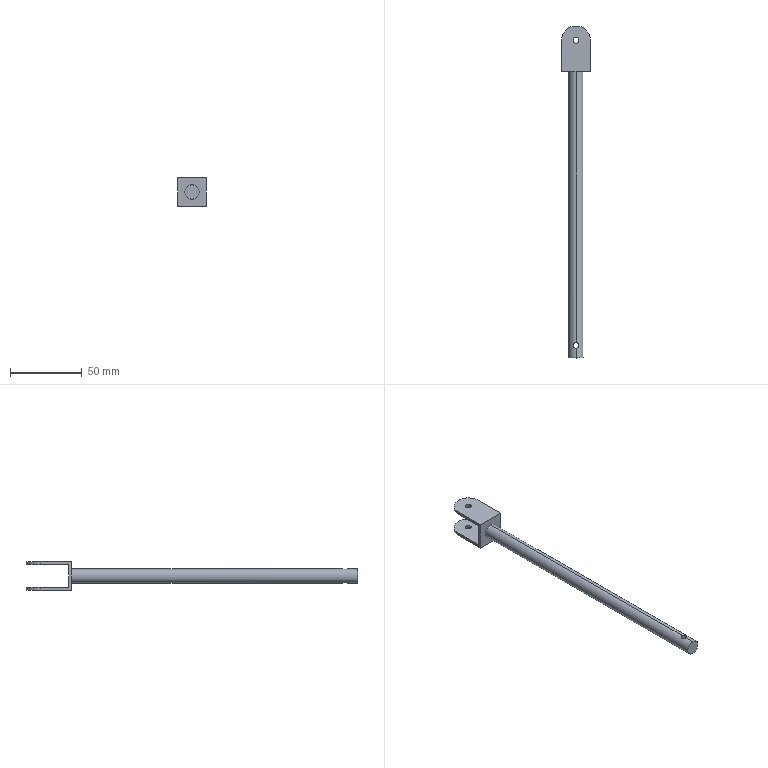Part | SolidWorks | features ICE 5, Extrusion 1 | 1 solid | 19 faces | box 20 x 232 x 20 mm | volume 18563 mm3 | cylinder 10 | plane 9 | commonest cylinder face diameters 4 x6 10 x2 20 x2
STEP:
#1=CARTESIAN_POINT('',(0.,-195.175,5.));
#2=VERTEX_POINT('',#1);
#3=CARTESIAN_POINT('',(2.,-193.175,4.583));
#4=VERTEX_POINT('',#3);
#5=CARTESIAN_POINT('',(0.,-195.175,5.));
#6=CARTESIAN_POINT('',(0.1337,-195.175,5.));
#7=CARTESIAN_POINT('',(0.2649,-195.162,4.995));
#8=CARTESIAN_POINT('',(0.5226,-195.11,4.974));
#9=CARTESIAN_POINT('',(0.6505,-195.071,4.959));
#10=CARTESIAN_POINT('',(0.8922,-194.97,4.921));
#11=CARTESIAN_POINT('',(1.007,-194.908,4.899));
#12=CARTESIAN_POINT('',(1.223,-194.763,4.849));
#13=CARTESIAN_POINT('',(1.324,-194.68,4.822));
#14=CARTESIAN_POINT('',(1.598,-194.405,4.742));
#15=CARTESIAN_POINT('',(1.746,-194.185,4.686));
#16=CARTESIAN_POINT('',(1.896,-193.825,4.627));
#17=CARTESIAN_POINT('',(1.935,-193.697,4.61));
#18=CARTESIAN_POINT('',(1.987,-193.438,4.588));
#19=CARTESIAN_POINT('',(2.,-193.307,4.583));
#20=CARTESIAN_POINT('',(2.,-193.175,4.583));
#21=B_SPLINE_CURVE_WITH_KNOTS('',3,(#5,#6,#7,#8,#9,#10,#11,#12,#13,#14,#15,#16,#17,#18,#19,#20),.UNSPECIFIED.,.F.,.F.,(4,2,2,2,2,2,2,4),(0.,0.0003951,0.0007903,0.001185,0.001581,0.002371,0.002766,0.003161),.UNSPECIFIED.);
#22=EDGE_CURVE('',#2,#4,#21,.T.);
#23=ORIENTED_EDGE('',*,*,#22,.T.);
#24=CARTESIAN_POINT('',(2.,-193.175,-4.583));
#25=VERTEX_POINT('',#24);
#26=CARTESIAN_POINT('',(2.,-193.175,30.5));
#27=DIRECTION('',(0.,0.,-1.));
#28=VECTOR('',#27,1000.);
#29=LINE('',#26,#28);
#30=EDGE_CURVE('',#4,#25,#29,.T.);
#31=ORIENTED_EDGE('',*,*,#30,.T.);
#32=CARTESIAN_POINT('',(0.,-195.175,-5.));
#33=VERTEX_POINT('',#32);
#34=CARTESIAN_POINT('',(2.,-193.175,-4.583));
#35=CARTESIAN_POINT('',(2.,-193.307,-4.583));
#36=CARTESIAN_POINT('',(1.987,-193.44,-4.588));
#37=CARTESIAN_POINT('',(1.935,-193.699,-4.611));
#38=CARTESIAN_POINT('',(1.896,-193.824,-4.627));
#39=CARTESIAN_POINT('',(1.795,-194.066,-4.667));
#40=CARTESIAN_POINT('',(1.733,-194.182,-4.691));
#41=CARTESIAN_POINT('',(1.589,-194.397,-4.742));
#42=CARTESIAN_POINT('',(1.506,-194.498,-4.769));
#43=CARTESIAN_POINT('',(1.322,-194.682,-4.823));
#44=CARTESIAN_POINT('',(1.222,-194.764,-4.85));
#45=CARTESIAN_POINT('',(1.007,-194.908,-4.899));
#46=CARTESIAN_POINT('',(0.8904,-194.971,-4.922));
#47=CARTESIAN_POINT('',(0.6487,-195.072,-4.959));
#48=CARTESIAN_POINT('',(0.5238,-195.11,-4.974));
#49=CARTESIAN_POINT('',(0.2659,-195.162,-4.995));
#50=CARTESIAN_POINT('',(0.1318,-195.175,-5.));
#51=CARTESIAN_POINT('',(0.,-195.175,-5.));
#52=B_SPLINE_CURVE_WITH_KNOTS('',3,(#34,#35,#36,#37,#38,#39,#40,#41,#42,#43,#44,#45,#46,#47,#48,#49,#50,#51),.UNSPECIFIED.,.F.,.F.,(4,2,2,2,2,2,2,2,4),(0.006319,0.006714,0.007109,0.007504,0.007898,0.008293,0.008688,0.009082,0.009477),.UNSPECIFIED.);
#53=EDGE_CURVE('',#25,#33,#52,.T.);
#54=ORIENTED_EDGE('',*,*,#53,.T.);
#55=CARTESIAN_POINT('',(-2.,-193.175,-4.583));
#56=VERTEX_POINT('',#55);
#57=CARTESIAN_POINT('',(0.,-195.175,-5.));
#58=CARTESIAN_POINT('',(-0.2635,-195.175,-5.));
#59=CARTESIAN_POINT('',(-0.5288,-195.122,-4.978));
#60=CARTESIAN_POINT('',(-0.8901,-194.971,-4.922));
#61=CARTESIAN_POINT('',(-1.007,-194.908,-4.899));
#62=CARTESIAN_POINT('',(-1.223,-194.763,-4.849));
#63=CARTESIAN_POINT('',(-1.322,-194.681,-4.823));
#64=CARTESIAN_POINT('',(-1.506,-194.498,-4.769));
#65=CARTESIAN_POINT('',(-1.589,-194.397,-4.741));
#66=CARTESIAN_POINT('',(-1.733,-194.182,-4.691));
#67=CARTESIAN_POINT('',(-1.794,-194.068,-4.667));
#68=CARTESIAN_POINT('',(-1.947,-193.704,-4.607));
#69=CARTESIAN_POINT('',(-2.,-193.442,-4.583));
#70=CARTESIAN_POINT('',(-2.,-193.175,-4.583));
#71=B_SPLINE_CURVE_WITH_KNOTS('',3,(#57,#58,#59,#60,#61,#62,#63,#64,#65,#66,#67,#68,#69,#70),.UNSPECIFIED.,.F.,.F.,(4,2,2,2,2,2,4),(0.009477,0.01027,0.01066,0.01106,0.01145,0.01184,0.01263),.UNSPECIFIED.);
#72=EDGE_CURVE('',#33,#56,#71,.T.);
#73=ORIENTED_EDGE('',*,*,#72,.T.);
#74=CARTESIAN_POINT('',(-2.,-193.175,4.583));
#75=VERTEX_POINT('',#74);
#76=CARTESIAN_POINT('',(-2.,-193.175,30.5));
#77=DIRECTION('',(0.,0.,-1.));
#78=VECTOR('',#77,1000.);
#79=LINE('',#76,#78);
#80=EDGE_CURVE('',#75,#56,#79,.T.);
#81=ORIENTED_EDGE('',*,*,#80,.F.);
#82=CARTESIAN_POINT('',(-2.,-193.175,4.583));
#83=CARTESIAN_POINT('',(-2.,-193.439,4.583));
#84=CARTESIAN_POINT('',(-1.946,-193.704,4.607));
#85=CARTESIAN_POINT('',(-1.796,-194.065,4.667));
#86=CARTESIAN_POINT('',(-1.733,-194.182,4.691));
#87=CARTESIAN_POINT('',(-1.588,-194.398,4.742));
#88=CARTESIAN_POINT('',(-1.506,-194.497,4.769));
#89=CARTESIAN_POINT('',(-1.323,-194.681,4.823));
#90=CARTESIAN_POINT('',(-1.222,-194.764,4.85));
#91=CARTESIAN_POINT('',(-1.007,-194.908,4.899));
#92=CARTESIAN_POINT('',(-0.8925,-194.97,4.921));
#93=CARTESIAN_POINT('',(-0.5272,-195.123,4.978));
#94=CARTESIAN_POINT('',(-0.2671,-195.175,5.));
#95=CARTESIAN_POINT('',(0.,-195.175,5.));
#96=B_SPLINE_CURVE_WITH_KNOTS('',3,(#82,#83,#84,#85,#86,#87,#88,#89,#90,#91,#92,#93,#94,#95),.UNSPECIFIED.,.F.,.F.,(4,2,2,2,2,2,4),(0.009478,0.01027,0.01066,0.01106,0.01145,0.01185,0.01264),.UNSPECIFIED.);
#97=EDGE_CURVE('',#75,#2,#96,.T.);
#98=ORIENTED_EDGE('',*,*,#97,.T.);
#99=EDGE_LOOP('',(#23,#31,#54,#73,#81,#98));
#100=FACE_OUTER_BOUND('',#99,.T.);
#101=CARTESIAN_POINT('',(0.,-193.175,30.5));
#102=DIRECTION('',(0.,0.,-1.));
#103=DIRECTION('',(-1.,0.,0.));
#104=AXIS2_PLACEMENT_3D('',#101,#102,#103);
#105=CYLINDRICAL_SURFACE('',#104,2.);
#106=ADVANCED_FACE('',(#100),#105,.F.);
#107=CARTESIAN_POINT('',(-2.,20.,10.));
#108=VERTEX_POINT('',#107);
#109=CARTESIAN_POINT('',(2.,20.,10.));
#110=VERTEX_POINT('',#109);
#111=CARTESIAN_POINT('',(0.,20.,10.));
#112=DIRECTION('',(0.,0.,1.));
#113=DIRECTION('',(1.,0.,0.));
#114=AXIS2_PLACEMENT_3D('',#111,#112,#113);
#115=CIRCLE('',#114,2.);
#116=EDGE_CURVE('',#108,#110,#115,.T.);
#117=ORIENTED_EDGE('',*,*,#116,.T.);
#118=CARTESIAN_POINT('',(2.,20.,8.));
#119=VERTEX_POINT('',#118);
#120=CARTESIAN_POINT('',(2.,20.,24.));
#121=DIRECTION('',(0.,0.,-1.));
#122=VECTOR('',#121,1000.);
#123=LINE('',#120,#122);
#124=EDGE_CURVE('',#110,#119,#123,.T.);
#125=ORIENTED_EDGE('',*,*,#124,.T.);
#126=CARTESIAN_POINT('',(-2.,20.,8.));
#127=VERTEX_POINT('',#126);
#128=CARTESIAN_POINT('',(0.,20.,8.));
#129=DIRECTION('',(0.,0.,-1.));
#130=DIRECTION('',(1.,0.,0.));
#131=AXIS2_PLACEMENT_3D('',#128,#129,#130);
#132=CIRCLE('',#131,2.);
#133=EDGE_CURVE('',#119,#127,#132,.T.);
#134=ORIENTED_EDGE('',*,*,#133,.T.);
#135=CARTESIAN_POINT('',(-2.,20.,24.));
#136=DIRECTION('',(0.,0.,-1.));
#137=VECTOR('',#136,1000.);
#138=LINE('',#135,#137);
#139=EDGE_CURVE('',#108,#127,#138,.T.);
#140=ORIENTED_EDGE('',*,*,#139,.F.);
#141=EDGE_LOOP('',(#117,#125,#134,#140));
#142=FACE_OUTER_BOUND('',#141,.T.);
#143=CARTESIAN_POINT('',(0.,20.,24.));
#144=DIRECTION('',(0.,0.,-1.));
#145=DIRECTION('',(-1.,0.,0.));
#146=AXIS2_PLACEMENT_3D('',#143,#144,#145);
#147=CYLINDRICAL_SURFACE('',#146,2.);
#148=ADVANCED_FACE('',(#142),#147,.F.);
#149=CARTESIAN_POINT('',(-2.,20.,-8.));
#150=VERTEX_POINT('',#149);
#151=CARTESIAN_POINT('',(2.,20.,-8.));
#152=VERTEX_POINT('',#151);
#153=CARTESIAN_POINT('',(0.,20.,-8.));
#154=DIRECTION('',(0.,0.,1.));
#155=DIRECTION('',(-1.,0.,0.));
#156=AXIS2_PLACEMENT_3D('',#153,#154,#155);
#157=CIRCLE('',#156,2.);
#158=EDGE_CURVE('',#150,#152,#157,.T.);
#159=ORIENTED_EDGE('',*,*,#158,.T.);
#160=CARTESIAN_POINT('',(2.,20.,-10.));
#161=VERTEX_POINT('',#160);
#162=CARTESIAN_POINT('',(2.,20.,24.));
#163=DIRECTION('',(0.,0.,-1.));
#164=VECTOR('',#163,1000.);
#165=LINE('',#162,#164);
#166=EDGE_CURVE('',#152,#161,#165,.T.);
#167=ORIENTED_EDGE('',*,*,#166,.T.);
#168=CARTESIAN_POINT('',(-2.,20.,-10.));
#169=VERTEX_POINT('',#168);
#170=CARTESIAN_POINT('',(0.,20.,-10.));
#171=DIRECTION('',(0.,0.,-1.));
#172=DIRECTION('',(-1.,0.,0.));
#173=AXIS2_PLACEMENT_3D('',#170,#171,#172);
#174=CIRCLE('',#173,2.);
#175=EDGE_CURVE('',#161,#169,#174,.T.);
#176=ORIENTED_EDGE('',*,*,#175,.T.);
#177=CARTESIAN_POINT('',(-2.,20.,24.));
#178=DIRECTION('',(0.,0.,-1.));
#179=VECTOR('',#178,1000.);
#180=LINE('',#177,#179);
#181=EDGE_CURVE('',#150,#169,#180,.T.);
#182=ORIENTED_EDGE('',*,*,#181,.F.);
#183=EDGE_LOOP('',(#159,#167,#176,#182));
#184=FACE_OUTER_BOUND('',#183,.T.);
#185=CARTESIAN_POINT('',(0.,20.,24.));
#186=DIRECTION('',(0.,0.,-1.));
#187=DIRECTION('',(-1.,0.,0.));
#188=AXIS2_PLACEMENT_3D('',#185,#186,#187);
#189=CYLINDRICAL_SURFACE('',#188,2.);
#190=ADVANCED_FACE('',(#184),#189,.F.);
#191=CARTESIAN_POINT('',(0.,-202.,-5.));
#192=VERTEX_POINT('',#191);
#193=CARTESIAN_POINT('',(0.,-202.,5.));
#194=VERTEX_POINT('',#193);
#195=CARTESIAN_POINT('',(0.,-202.,0.));
#196=DIRECTION('',(0.,-1.,0.));
#197=DIRECTION('',(0.,0.,-1.));
#198=AXIS2_PLACEMENT_3D('',#195,#196,#197);
#199=CIRCLE('',#198,5.);
#200=EDGE_CURVE('',#192,#194,#199,.T.);
#201=ORIENTED_EDGE('',*,*,#200,.F.);
#202=CARTESIAN_POINT('',(0.,-202.,-5.));
#203=DIRECTION('',(0.,1.,0.));
#204=VECTOR('',#203,1000.);
#205=LINE('',#202,#204);
#206=EDGE_CURVE('',#192,#33,#205,.T.);
#207=ORIENTED_EDGE('',*,*,#206,.T.);
#208=ORIENTED_EDGE('',*,*,#53,.F.);
#209=CARTESIAN_POINT('',(0.,-191.175,-5.));
#210=VERTEX_POINT('',#209);
#211=CARTESIAN_POINT('',(0.,-191.175,-5.));
#212=CARTESIAN_POINT('',(0.1321,-191.175,-5.));
#213=CARTESIAN_POINT('',(0.266,-191.189,-4.995));
#214=CARTESIAN_POINT('',(0.5238,-191.241,-4.974));
#215=CARTESIAN_POINT('',(0.6494,-191.279,-4.959));
#216=CARTESIAN_POINT('',(0.8932,-191.381,-4.921));
#217=CARTESIAN_POINT('',(1.008,-191.443,-4.899));
#218=CARTESIAN_POINT('',(1.223,-191.587,-4.849));
#219=CARTESIAN_POINT('',(1.325,-191.671,-4.822));
#220=CARTESIAN_POINT('',(1.507,-191.854,-4.768));
#221=CARTESIAN_POINT('',(1.589,-191.954,-4.741));
#222=CARTESIAN_POINT('',(1.734,-192.17,-4.69));
#223=CARTESIAN_POINT('',(1.796,-192.286,-4.666));
#224=CARTESIAN_POINT('',(1.946,-192.647,-4.607));
#225=CARTESIAN_POINT('',(2.,-192.912,-4.583));
#226=CARTESIAN_POINT('',(2.,-193.175,-4.583));
#227=B_SPLINE_CURVE_WITH_KNOTS('',3,(#211,#212,#213,#214,#215,#216,#217,#218,#219,#220,#221,#222,#223,#224,#225,#226),.UNSPECIFIED.,.F.,.F.,(4,2,2,2,2,2,2,4),(0.003161,0.003556,0.00395,0.004345,0.00474,0.005135,0.00553,0.006319),.UNSPECIFIED.);
#228=EDGE_CURVE('',#210,#25,#227,.T.);
#229=ORIENTED_EDGE('',*,*,#228,.F.);
#230=CARTESIAN_POINT('',(0.,-2.,-5.));
#231=VERTEX_POINT('',#230);
#232=CARTESIAN_POINT('',(0.,-202.,-5.));
#233=DIRECTION('',(0.,1.,0.));
#234=VECTOR('',#233,1000.);
#235=LINE('',#232,#234);
#236=EDGE_CURVE('',#210,#231,#235,.T.);
#237=ORIENTED_EDGE('',*,*,#236,.T.);
#238=CARTESIAN_POINT('',(0.,-2.,5.));
#239=VERTEX_POINT('',#238);
#240=CARTESIAN_POINT('',(0.,-2.,0.));
#241=DIRECTION('',(0.,-1.,0.));
#242=DIRECTION('',(0.,0.,-1.));
#243=AXIS2_PLACEMENT_3D('',#240,#241,#242);
#244=CIRCLE('',#243,5.);
#245=EDGE_CURVE('',#231,#239,#244,.T.);
#246=ORIENTED_EDGE('',*,*,#245,.T.);
#247=CARTESIAN_POINT('',(0.,-191.175,5.));
#248=VERTEX_POINT('',#247);
#249=CARTESIAN_POINT('',(0.,-202.,5.));
#250=DIRECTION('',(0.,1.,0.));
#251=VECTOR('',#250,1000.);
#252=LINE('',#249,#251);
#253=EDGE_CURVE('',#248,#239,#252,.T.);
#254=ORIENTED_EDGE('',*,*,#253,.F.);
#255=CARTESIAN_POINT('',(2.,-193.175,4.583));
#256=CARTESIAN_POINT('',(2.,-193.043,4.583));
#257=CARTESIAN_POINT('',(1.987,-192.909,4.588));
#258=CARTESIAN_POINT('',(1.935,-192.652,4.611));
#259=CARTESIAN_POINT('',(1.896,-192.526,4.627));
#260=CARTESIAN_POINT('',(1.795,-192.283,4.667));
#261=CARTESIAN_POINT('',(1.733,-192.168,4.691));
#262=CARTESIAN_POINT('',(1.588,-191.953,4.742));
#263=CARTESIAN_POINT('',(1.505,-191.852,4.769));
#264=CARTESIAN_POINT('',(1.322,-191.669,4.823));
#265=CARTESIAN_POINT('',(1.222,-191.587,4.85));
#266=CARTESIAN_POINT('',(1.006,-191.442,4.899));
#267=CARTESIAN_POINT('',(0.8895,-191.379,4.922));
#268=CARTESIAN_POINT('',(0.5289,-191.229,4.978));
#269=CARTESIAN_POINT('',(0.2632,-191.175,5.));
#270=CARTESIAN_POINT('',(0.,-191.175,5.));
#271=B_SPLINE_CURVE_WITH_KNOTS('',3,(#255,#256,#257,#258,#259,#260,#261,#262,#263,#264,#265,#266,#267,#268,#269,#270),.UNSPECIFIED.,.F.,.F.,(4,2,2,2,2,2,2,4),(0.003161,0.003556,0.003951,0.004346,0.00474,0.005135,0.00553,0.00632),.UNSPECIFIED.);
#272=EDGE_CURVE('',#4,#248,#271,.T.);
#273=ORIENTED_EDGE('',*,*,#272,.F.);
#274=ORIENTED_EDGE('',*,*,#22,.F.);
#275=CARTESIAN_POINT('',(0.,-202.,5.));
#276=DIRECTION('',(0.,1.,0.));
#277=VECTOR('',#276,1000.);
#278=LINE('',#275,#277);
#279=EDGE_CURVE('',#194,#2,#278,.T.);
#280=ORIENTED_EDGE('',*,*,#279,.F.);
#281=EDGE_LOOP('',(#201,#207,#208,#229,#237,#246,#254,#273,#274,#280));
#282=FACE_OUTER_BOUND('',#281,.T.);
#283=CARTESIAN_POINT('',(0.,-202.,0.));
#284=DIRECTION('',(0.,1.,0.));
#285=DIRECTION('',(0.,0.,1.));
#286=AXIS2_PLACEMENT_3D('',#283,#284,#285);
#287=CYLINDRICAL_SURFACE('',#286,5.);
#288=ADVANCED_FACE('',(#282),#287,.T.);
#289=ORIENTED_EDGE('',*,*,#206,.F.);
#290=CARTESIAN_POINT('',(0.,-202.,0.));
#291=DIRECTION('',(0.,-1.,0.));
#292=DIRECTION('',(0.,0.,-1.));
#293=AXIS2_PLACEMENT_3D('',#290,#291,#292);
#294=CIRCLE('',#293,5.);
#295=EDGE_CURVE('',#194,#192,#294,.T.);
#296=ORIENTED_EDGE('',*,*,#295,.F.);
#297=ORIENTED_EDGE('',*,*,#279,.T.);
#298=ORIENTED_EDGE('',*,*,#97,.F.);
#299=CARTESIAN_POINT('',(0.,-191.175,5.));
#300=CARTESIAN_POINT('',(-0.1316,-191.175,5.));
#301=CARTESIAN_POINT('',(-0.2649,-191.189,4.995));
#302=CARTESIAN_POINT('',(-0.5241,-191.241,4.974));
#303=CARTESIAN_POINT('',(-0.6493,-191.279,4.959));
#304=CARTESIAN_POINT('',(-0.8913,-191.38,4.921));
#305=CARTESIAN_POINT('',(-1.008,-191.443,4.899));
#306=CARTESIAN_POINT('',(-1.223,-191.587,4.849));
#307=CARTESIAN_POINT('',(-1.323,-191.67,4.823));
#308=CARTESIAN_POINT('',(-1.508,-191.855,4.768));
#309=CARTESIAN_POINT('',(-1.589,-191.954,4.741));
#310=CARTESIAN_POINT('',(-1.733,-192.169,4.691));
#311=CARTESIAN_POINT('',(-1.796,-192.285,4.667));
#312=CARTESIAN_POINT('',(-1.897,-192.527,4.627));
#313=CARTESIAN_POINT('',(-1.935,-192.652,4.611));
#314=CARTESIAN_POINT('',(-1.987,-192.909,4.588));
#315=CARTESIAN_POINT('',(-2.,-193.043,4.583));
#316=CARTESIAN_POINT('',(-2.,-193.175,4.583));
#317=B_SPLINE_CURVE_WITH_KNOTS('',3,(#299,#300,#301,#302,#303,#304,#305,#306,#307,#308,#309,#310,#311,#312,#313,#314,#315,#316),.UNSPECIFIED.,.F.,.F.,(4,2,2,2,2,2,2,2,4),(0.00632,0.006715,0.007109,0.007504,0.007899,0.008294,0.008688,0.009083,0.009478),.UNSPECIFIED.);
#318=EDGE_CURVE('',#248,#75,#317,.T.);
#319=ORIENTED_EDGE('',*,*,#318,.F.);
#320=ORIENTED_EDGE('',*,*,#253,.T.);
#321=CARTESIAN_POINT('',(0.,-2.,0.));
#322=DIRECTION('',(0.,-1.,0.));
#323=DIRECTION('',(0.,0.,-1.));
#324=AXIS2_PLACEMENT_3D('',#321,#322,#323);
#325=CIRCLE('',#324,5.);
#326=EDGE_CURVE('',#239,#231,#325,.T.);
#327=ORIENTED_EDGE('',*,*,#326,.T.);
#328=ORIENTED_EDGE('',*,*,#236,.F.);
#329=CARTESIAN_POINT('',(-2.,-193.175,-4.583));
#330=CARTESIAN_POINT('',(-2.,-193.042,-4.583));
#331=CARTESIAN_POINT('',(-1.987,-192.91,-4.588));
#332=CARTESIAN_POINT('',(-1.935,-192.653,-4.61));
#333=CARTESIAN_POINT('',(-1.896,-192.525,-4.627));
#334=CARTESIAN_POINT('',(-1.795,-192.284,-4.667));
#335=CARTESIAN_POINT('',(-1.734,-192.169,-4.691));
#336=CARTESIAN_POINT('',(-1.588,-191.953,-4.742));
#337=CARTESIAN_POINT('',(-1.505,-191.852,-4.769));
#338=CARTESIAN_POINT('',(-1.231,-191.578,-4.85));
#339=CARTESIAN_POINT('',(-1.01,-191.43,-4.903));
#340=CARTESIAN_POINT('',(-0.6497,-191.279,-4.959));
#341=CARTESIAN_POINT('',(-0.522,-191.24,-4.974));
#342=CARTESIAN_POINT('',(-0.263,-191.188,-4.995));
#343=CARTESIAN_POINT('',(-0.1322,-191.175,-5.));
#344=CARTESIAN_POINT('',(0.,-191.175,-5.));
#345=B_SPLINE_CURVE_WITH_KNOTS('',3,(#329,#330,#331,#332,#333,#334,#335,#336,#337,#338,#339,#340,#341,#342,#343,#344),.UNSPECIFIED.,.F.,.F.,(4,2,2,2,2,2,2,4),(0.,0.0003951,0.0007902,0.001185,0.00158,0.002371,0.002766,0.003161),.UNSPECIFIED.);
#346=EDGE_CURVE('',#56,#210,#345,.T.);
#347=ORIENTED_EDGE('',*,*,#346,.F.);
#348=ORIENTED_EDGE('',*,*,#72,.F.);
#349=EDGE_LOOP('',(#289,#296,#297,#298,#319,#320,#327,#328,#347,#348));
#350=FACE_OUTER_BOUND('',#349,.T.);
#351=CARTESIAN_POINT('',(0.,-202.,0.));
#352=DIRECTION('',(0.,1.,0.));
#353=DIRECTION('',(0.,0.,1.));
#354=AXIS2_PLACEMENT_3D('',#351,#352,#353);
#355=CYLINDRICAL_SURFACE('',#354,5.);
#356=ADVANCED_FACE('',(#350),#355,.T.);
#357=CARTESIAN_POINT('',(-10.,0.,8.));
#358=VERTEX_POINT('',#357);
#359=CARTESIAN_POINT('',(-10.,0.,-8.));
#360=VERTEX_POINT('',#359);
#361=CARTESIAN_POINT('',(-10.,0.,-10.));
#362=DIRECTION('',(0.,0.,-1.));
#363=VECTOR('',#362,1000.);
#364=LINE('',#361,#363);
#365=EDGE_CURVE('',#358,#360,#364,.T.);
#366=ORIENTED_EDGE('',*,*,#365,.F.);
#367=CARTESIAN_POINT('',(10.,0.,8.));
#368=VERTEX_POINT('',#367);
#369=CARTESIAN_POINT('',(-10.,0.,8.));
#370=DIRECTION('',(1.,0.,0.));
#371=VECTOR('',#370,1000.);
#372=LINE('',#369,#371);
#373=EDGE_CURVE('',#358,#368,#372,.T.);
#374=ORIENTED_EDGE('',*,*,#373,.T.);
#375=CARTESIAN_POINT('',(10.,0.,-8.));
#376=VERTEX_POINT('',#375);
#377=CARTESIAN_POINT('',(10.,0.,-10.));
#378=DIRECTION('',(0.,0.,1.));
#379=VECTOR('',#378,1000.);
#380=LINE('',#377,#379);
#381=EDGE_CURVE('',#376,#368,#380,.T.);
#382=ORIENTED_EDGE('',*,*,#381,.F.);
#383=CARTESIAN_POINT('',(-10.,0.,-8.));
#384=DIRECTION('',(-1.,0.,0.));
#385=VECTOR('',#384,1000.);
#386=LINE('',#383,#385);
#387=EDGE_CURVE('',#376,#360,#386,.T.);
#388=ORIENTED_EDGE('',*,*,#387,.T.);
#389=EDGE_LOOP('',(#366,#374,#382,#388));
#390=FACE_OUTER_BOUND('',#389,.T.);
#391=CARTESIAN_POINT('',(0.,0.,0.));
#392=DIRECTION('',(0.,1.,0.));
#393=DIRECTION('',(0.,0.,1.));
#394=AXIS2_PLACEMENT_3D('',#391,#392,#393);
#395=PLANE('',#394);
#396=ADVANCED_FACE('',(#390),#395,.T.);
#397=CARTESIAN_POINT('',(-10.,20.,-8.));
#398=VERTEX_POINT('',#397);
#399=CARTESIAN_POINT('',(-10.,20.,-10.));
#400=VERTEX_POINT('',#399);
#401=CARTESIAN_POINT('',(-10.,20.,10.));
#402=DIRECTION('',(0.,0.,-1.));
#403=VECTOR('',#402,1000.);
#404=LINE('',#401,#403);
#405=EDGE_CURVE('',#398,#400,#404,.T.);
#406=ORIENTED_EDGE('',*,*,#405,.F.);
#407=CARTESIAN_POINT('',(10.,20.,-8.));
#408=VERTEX_POINT('',#407);
#409=CARTESIAN_POINT('',(0.,20.,-8.));
#410=DIRECTION('',(0.,0.,-1.));
#411=DIRECTION('',(-1.,0.,0.));
#412=AXIS2_PLACEMENT_3D('',#409,#410,#411);
#413=CIRCLE('',#412,10.);
#414=EDGE_CURVE('',#398,#408,#413,.T.);
#415=ORIENTED_EDGE('',*,*,#414,.T.);
#416=CARTESIAN_POINT('',(10.,20.,-10.));
#417=VERTEX_POINT('',#416);
#418=CARTESIAN_POINT('',(10.,20.,10.));
#419=DIRECTION('',(0.,0.,-1.));
#420=VECTOR('',#419,1000.);
#421=LINE('',#418,#420);
#422=EDGE_CURVE('',#408,#417,#421,.T.);
#423=ORIENTED_EDGE('',*,*,#422,.T.);
#424=CARTESIAN_POINT('',(0.,20.,-10.));
#425=DIRECTION('',(0.,0.,1.));
#426=DIRECTION('',(1.,0.,0.));
#427=AXIS2_PLACEMENT_3D('',#424,#425,#426);
#428=CIRCLE('',#427,10.);
#429=EDGE_CURVE('',#417,#400,#428,.T.);
#430=ORIENTED_EDGE('',*,*,#429,.T.);
#431=EDGE_LOOP('',(#406,#415,#423,#430));
#432=FACE_OUTER_BOUND('',#431,.T.);
#433=CARTESIAN_POINT('',(0.,20.,10.));
#434=DIRECTION('',(0.,0.,-1.));
#435=DIRECTION('',(-1.,0.,0.));
#436=AXIS2_PLACEMENT_3D('',#433,#434,#435);
#437=CYLINDRICAL_SURFACE('',#436,10.);
#438=ADVANCED_FACE('',(#432),#437,.T.);
#439=CARTESIAN_POINT('',(-10.,-2.,-10.));
#440=VERTEX_POINT('',#439);
#441=CARTESIAN_POINT('',(-10.,20.,-10.));
#442=DIRECTION('',(0.,-1.,0.));
#443=VECTOR('',#442,1000.);
#444=LINE('',#441,#443);
#445=EDGE_CURVE('',#400,#440,#444,.T.);
#446=ORIENTED_EDGE('',*,*,#445,.T.);
#447=CARTESIAN_POINT('',(-10.,-2.,10.));
#448=VERTEX_POINT('',#447);
#449=CARTESIAN_POINT('',(-10.,-2.,-10.));
#450=DIRECTION('',(0.,0.,-1.));
#451=VECTOR('',#450,1000.);
#452=LINE('',#449,#451);
#453=EDGE_CURVE('',#448,#440,#452,.T.);
#454=ORIENTED_EDGE('',*,*,#453,.F.);
#455=CARTESIAN_POINT('',(-10.,20.,10.));
#456=VERTEX_POINT('',#455);
#457=CARTESIAN_POINT('',(-10.,-2.,10.));
#458=DIRECTION('',(0.,1.,0.));
#459=VECTOR('',#458,1000.);
#460=LINE('',#457,#459);
#461=EDGE_CURVE('',#448,#456,#460,.T.);
#462=ORIENTED_EDGE('',*,*,#461,.T.);
#463=CARTESIAN_POINT('',(-10.,20.,8.));
#464=VERTEX_POINT('',#463);
#465=CARTESIAN_POINT('',(-10.,20.,10.));
#466=DIRECTION('',(0.,0.,-1.));
#467=VECTOR('',#466,1000.);
#468=LINE('',#465,#467);
#469=EDGE_CURVE('',#456,#464,#468,.T.);
#470=ORIENTED_EDGE('',*,*,#469,.T.);
#471=CARTESIAN_POINT('',(-10.,20.,8.));
#472=DIRECTION('',(0.,-1.,0.));
#473=VECTOR('',#472,1000.);
#474=LINE('',#471,#473);
#475=EDGE_CURVE('',#464,#358,#474,.T.);
#476=ORIENTED_EDGE('',*,*,#475,.T.);
#477=ORIENTED_EDGE('',*,*,#365,.T.);
#478=CARTESIAN_POINT('',(-10.,20.,-8.));
#479=DIRECTION('',(0.,1.,0.));
#480=VECTOR('',#479,1000.);
#481=LINE('',#478,#480);
#482=EDGE_CURVE('',#360,#398,#481,.T.);
#483=ORIENTED_EDGE('',*,*,#482,.T.);
#484=ORIENTED_EDGE('',*,*,#405,.T.);
#485=EDGE_LOOP('',(#446,#454,#462,#470,#476,#477,#483,#484));
#486=FACE_OUTER_BOUND('',#485,.T.);
#487=CARTESIAN_POINT('',(-10.,20.,10.));
#488=DIRECTION('',(1.,0.,0.));
#489=DIRECTION('',(0.,1.,0.));
#490=AXIS2_PLACEMENT_3D('',#487,#488,#489);
#491=PLANE('',#490);
#492=ADVANCED_FACE('',(#486),#491,.F.);
#493=ORIENTED_EDGE('',*,*,#422,.F.);
#494=CARTESIAN_POINT('',(10.,0.,-8.));
#495=DIRECTION('',(0.,-1.,0.));
#496=VECTOR('',#495,1000.);
#497=LINE('',#494,#496);
#498=EDGE_CURVE('',#408,#376,#497,.T.);
#499=ORIENTED_EDGE('',*,*,#498,.T.);
#500=ORIENTED_EDGE('',*,*,#381,.T.);
#501=CARTESIAN_POINT('',(10.,20.,8.));
#502=VERTEX_POINT('',#501);
#503=CARTESIAN_POINT('',(10.,0.,8.));
#504=DIRECTION('',(0.,1.,0.));
#505=VECTOR('',#504,1000.);
#506=LINE('',#503,#505);
#507=EDGE_CURVE('',#368,#502,#506,.T.);
#508=ORIENTED_EDGE('',*,*,#507,.T.);
#509=CARTESIAN_POINT('',(10.,20.,10.));
#510=VERTEX_POINT('',#509);
#511=CARTESIAN_POINT('',(10.,20.,10.));
#512=DIRECTION('',(0.,0.,-1.));
#513=VECTOR('',#512,1000.);
#514=LINE('',#511,#513);
#515=EDGE_CURVE('',#510,#502,#514,.T.);
#516=ORIENTED_EDGE('',*,*,#515,.F.);
#517=CARTESIAN_POINT('',(10.,-2.,10.));
#518=VERTEX_POINT('',#517);
#519=CARTESIAN_POINT('',(10.,-2.,10.));
#520=DIRECTION('',(0.,1.,0.));
#521=VECTOR('',#520,1000.);
#522=LINE('',#519,#521);
#523=EDGE_CURVE('',#518,#510,#522,.T.);
#524=ORIENTED_EDGE('',*,*,#523,.F.);
#525=CARTESIAN_POINT('',(10.,-2.,-10.));
#526=VERTEX_POINT('',#525);
#527=CARTESIAN_POINT('',(10.,-2.,-10.));
#528=DIRECTION('',(0.,0.,1.));
#529=VECTOR('',#528,1000.);
#530=LINE('',#527,#529);
#531=EDGE_CURVE('',#526,#518,#530,.T.);
#532=ORIENTED_EDGE('',*,*,#531,.F.);
#533=CARTESIAN_POINT('',(10.,0.,-10.));
#534=DIRECTION('',(0.,1.,0.));
#535=VECTOR('',#534,1000.);
#536=LINE('',#533,#535);
#537=EDGE_CURVE('',#526,#417,#536,.T.);
#538=ORIENTED_EDGE('',*,*,#537,.T.);
#539=EDGE_LOOP('',(#493,#499,#500,#508,#516,#524,#532,#538));
#540=FACE_OUTER_BOUND('',#539,.T.);
#541=CARTESIAN_POINT('',(10.,0.,10.));
#542=DIRECTION('',(-1.,0.,0.));
#543=DIRECTION('',(0.,-1.,0.));
#544=AXIS2_PLACEMENT_3D('',#541,#542,#543);
#545=PLANE('',#544);
#546=ADVANCED_FACE('',(#540),#545,.F.);
#547=ORIENTED_EDGE('',*,*,#166,.F.);
#548=CARTESIAN_POINT('',(0.,20.,-8.));
#549=DIRECTION('',(0.,0.,1.));
#550=DIRECTION('',(-1.,0.,0.));
#551=AXIS2_PLACEMENT_3D('',#548,#549,#550);
#552=CIRCLE('',#551,2.);
#553=EDGE_CURVE('',#152,#150,#552,.T.);
#554=ORIENTED_EDGE('',*,*,#553,.T.);
#555=ORIENTED_EDGE('',*,*,#181,.T.);
#556=CARTESIAN_POINT('',(0.,20.,-10.));
#557=DIRECTION('',(0.,0.,-1.));
#558=DIRECTION('',(-1.,0.,0.));
#559=AXIS2_PLACEMENT_3D('',#556,#557,#558);
#560=CIRCLE('',#559,2.);
#561=EDGE_CURVE('',#169,#161,#560,.T.);
#562=ORIENTED_EDGE('',*,*,#561,.T.);
#563=EDGE_LOOP('',(#547,#554,#555,#562));
#564=FACE_OUTER_BOUND('',#563,.T.);
#565=CARTESIAN_POINT('',(0.,20.,24.));
#566=DIRECTION('',(0.,0.,-1.));
#567=DIRECTION('',(-1.,0.,0.));
#568=AXIS2_PLACEMENT_3D('',#565,#566,#567);
#569=CYLINDRICAL_SURFACE('',#568,2.);
#570=ADVANCED_FACE('',(#564),#569,.F.);
#571=ORIENTED_EDGE('',*,*,#561,.F.);
#572=ORIENTED_EDGE('',*,*,#175,.F.);
#573=EDGE_LOOP('',(#571,#572));
#574=FACE_BOUND('',#573,.T.);
#575=ORIENTED_EDGE('',*,*,#429,.F.);
#576=ORIENTED_EDGE('',*,*,#537,.F.);
#577=CARTESIAN_POINT('',(-10.,-2.,-10.));
#578=DIRECTION('',(1.,0.,0.));
#579=VECTOR('',#578,1000.);
#580=LINE('',#577,#579);
#581=EDGE_CURVE('',#440,#526,#580,.T.);
#582=ORIENTED_EDGE('',*,*,#581,.F.);
#583=ORIENTED_EDGE('',*,*,#445,.F.);
#584=EDGE_LOOP('',(#575,#576,#582,#583));
#585=FACE_OUTER_BOUND('',#584,.T.);
#586=CARTESIAN_POINT('',(0.,20.,-10.));
#587=DIRECTION('',(0.,0.,1.));
#588=DIRECTION('',(1.,0.,0.));
#589=AXIS2_PLACEMENT_3D('',#586,#587,#588);
#590=PLANE('',#589);
#591=ADVANCED_FACE('',(#574,#585),#590,.F.);
#592=ORIENTED_EDGE('',*,*,#158,.F.);
#593=ORIENTED_EDGE('',*,*,#553,.F.);
#594=EDGE_LOOP('',(#592,#593));
#595=FACE_BOUND('',#594,.T.);
#596=ORIENTED_EDGE('',*,*,#482,.F.);
#597=ORIENTED_EDGE('',*,*,#387,.F.);
#598=ORIENTED_EDGE('',*,*,#498,.F.);
#599=ORIENTED_EDGE('',*,*,#414,.F.);
#600=EDGE_LOOP('',(#596,#597,#598,#599));
#601=FACE_OUTER_BOUND('',#600,.T.);
#602=CARTESIAN_POINT('',(-17.,-43.929,-8.));
#603=DIRECTION('',(0.,0.,-1.));
#604=DIRECTION('',(-1.,0.,0.));
#605=AXIS2_PLACEMENT_3D('',#602,#603,#604);
#606=PLANE('',#605);
#607=ADVANCED_FACE('',(#595,#601),#606,.F.);
#608=ORIENTED_EDGE('',*,*,#523,.T.);
#609=CARTESIAN_POINT('',(0.,20.,10.));
#610=DIRECTION('',(0.,0.,1.));
#611=DIRECTION('',(1.,0.,0.));
#612=AXIS2_PLACEMENT_3D('',#609,#610,#611);
#613=CIRCLE('',#612,10.);
#614=EDGE_CURVE('',#510,#456,#613,.T.);
#615=ORIENTED_EDGE('',*,*,#614,.T.);
#616=ORIENTED_EDGE('',*,*,#461,.F.);
#617=CARTESIAN_POINT('',(-10.,-2.,10.));
#618=DIRECTION('',(-1.,0.,0.));
#619=VECTOR('',#618,1000.);
#620=LINE('',#617,#619);
#621=EDGE_CURVE('',#518,#448,#620,.T.);
#622=ORIENTED_EDGE('',*,*,#621,.F.);
#623=EDGE_LOOP('',(#608,#615,#616,#622));
#624=FACE_OUTER_BOUND('',#623,.T.);
#625=ORIENTED_EDGE('',*,*,#116,.F.);
#626=CARTESIAN_POINT('',(0.,20.,10.));
#627=DIRECTION('',(0.,0.,1.));
#628=DIRECTION('',(1.,0.,0.));
#629=AXIS2_PLACEMENT_3D('',#626,#627,#628);
#630=CIRCLE('',#629,2.);
#631=EDGE_CURVE('',#110,#108,#630,.T.);
#632=ORIENTED_EDGE('',*,*,#631,.F.);
#633=EDGE_LOOP('',(#625,#632));
#634=FACE_BOUND('',#633,.T.);
#635=CARTESIAN_POINT('',(-10.,-2.,10.));
#636=DIRECTION('',(0.,0.,-1.));
#637=DIRECTION('',(-1.,0.,0.));
#638=AXIS2_PLACEMENT_3D('',#635,#636,#637);
#639=PLANE('',#638);
#640=ADVANCED_FACE('',(#624,#634),#639,.F.);
#641=ORIENTED_EDGE('',*,*,#326,.F.);
#642=ORIENTED_EDGE('',*,*,#245,.F.);
#643=EDGE_LOOP('',(#641,#642));
#644=FACE_BOUND('',#643,.T.);
#645=ORIENTED_EDGE('',*,*,#531,.T.);
#646=ORIENTED_EDGE('',*,*,#621,.T.);
#647=ORIENTED_EDGE('',*,*,#453,.T.);
#648=ORIENTED_EDGE('',*,*,#581,.T.);
#649=EDGE_LOOP('',(#645,#646,#647,#648));
#650=FACE_OUTER_BOUND('',#649,.T.);
#651=CARTESIAN_POINT('',(0.,-2.,0.));
#652=DIRECTION('',(0.,1.,0.));
#653=DIRECTION('',(0.,0.,1.));
#654=AXIS2_PLACEMENT_3D('',#651,#652,#653);
#655=PLANE('',#654);
#656=ADVANCED_FACE('',(#644,#650),#655,.F.);
#657=ORIENTED_EDGE('',*,*,#515,.T.);
#658=CARTESIAN_POINT('',(0.,20.,8.));
#659=DIRECTION('',(0.,0.,1.));
#660=DIRECTION('',(1.,0.,0.));
#661=AXIS2_PLACEMENT_3D('',#658,#659,#660);
#662=CIRCLE('',#661,10.);
#663=EDGE_CURVE('',#502,#464,#662,.T.);
#664=ORIENTED_EDGE('',*,*,#663,.T.);
#665=ORIENTED_EDGE('',*,*,#469,.F.);
#666=ORIENTED_EDGE('',*,*,#614,.F.);
#667=EDGE_LOOP('',(#657,#664,#665,#666));
#668=FACE_OUTER_BOUND('',#667,.T.);
#669=CARTESIAN_POINT('',(0.,20.,10.));
#670=DIRECTION('',(0.,0.,-1.));
#671=DIRECTION('',(-1.,0.,0.));
#672=AXIS2_PLACEMENT_3D('',#669,#670,#671);
#673=CYLINDRICAL_SURFACE('',#672,10.);
#674=ADVANCED_FACE('',(#668),#673,.T.);
#675=ORIENTED_EDGE('',*,*,#124,.F.);
#676=ORIENTED_EDGE('',*,*,#631,.T.);
#677=ORIENTED_EDGE('',*,*,#139,.T.);
#678=CARTESIAN_POINT('',(0.,20.,8.));
#679=DIRECTION('',(0.,0.,-1.));
#680=DIRECTION('',(1.,0.,0.));
#681=AXIS2_PLACEMENT_3D('',#678,#679,#680);
#682=CIRCLE('',#681,2.);
#683=EDGE_CURVE('',#127,#119,#682,.T.);
#684=ORIENTED_EDGE('',*,*,#683,.T.);
#685=EDGE_LOOP('',(#675,#676,#677,#684));
#686=FACE_OUTER_BOUND('',#685,.T.);
#687=CARTESIAN_POINT('',(0.,20.,24.));
#688=DIRECTION('',(0.,0.,-1.));
#689=DIRECTION('',(-1.,0.,0.));
#690=AXIS2_PLACEMENT_3D('',#687,#688,#689);
#691=CYLINDRICAL_SURFACE('',#690,2.);
#692=ADVANCED_FACE('',(#686),#691,.F.);
#693=ORIENTED_EDGE('',*,*,#683,.F.);
#694=ORIENTED_EDGE('',*,*,#133,.F.);
#695=EDGE_LOOP('',(#693,#694));
#696=FACE_BOUND('',#695,.T.);
#697=ORIENTED_EDGE('',*,*,#507,.F.);
#698=ORIENTED_EDGE('',*,*,#373,.F.);
#699=ORIENTED_EDGE('',*,*,#475,.F.);
#700=ORIENTED_EDGE('',*,*,#663,.F.);
#701=EDGE_LOOP('',(#697,#698,#699,#700));
#702=FACE_OUTER_BOUND('',#701,.T.);
#703=CARTESIAN_POINT('',(-17.,-43.929,8.));
#704=DIRECTION('',(0.,0.,1.));
#705=DIRECTION('',(1.,0.,0.));
#706=AXIS2_PLACEMENT_3D('',#703,#704,#705);
#707=PLANE('',#706);
#708=ADVANCED_FACE('',(#696,#702),#707,.F.);
#709=ORIENTED_EDGE('',*,*,#295,.T.);
#710=ORIENTED_EDGE('',*,*,#200,.T.);
#711=EDGE_LOOP('',(#709,#710));
#712=FACE_OUTER_BOUND('',#711,.T.);
#713=CARTESIAN_POINT('',(0.,-202.,0.));
#714=DIRECTION('',(0.,-1.,0.));
#715=DIRECTION('',(0.,0.,-1.));
#716=AXIS2_PLACEMENT_3D('',#713,#714,#715);
#717=PLANE('',#716);
#718=ADVANCED_FACE('',(#712),#717,.T.);
#719=ORIENTED_EDGE('',*,*,#30,.F.);
#720=ORIENTED_EDGE('',*,*,#272,.T.);
#721=ORIENTED_EDGE('',*,*,#318,.T.);
#722=ORIENTED_EDGE('',*,*,#80,.T.);
#723=ORIENTED_EDGE('',*,*,#346,.T.);
#724=ORIENTED_EDGE('',*,*,#228,.T.);
#725=EDGE_LOOP('',(#719,#720,#721,#722,#723,#724));
#726=FACE_OUTER_BOUND('',#725,.T.);
#727=CARTESIAN_POINT('',(0.,-193.175,30.5));
#728=DIRECTION('',(0.,0.,-1.));
#729=DIRECTION('',(-1.,0.,0.));
#730=AXIS2_PLACEMENT_3D('',#727,#728,#729);
#731=CYLINDRICAL_SURFACE('',#730,2.);
#732=ADVANCED_FACE('',(#726),#731,.F.);
#733=CLOSED_SHELL('',(#106,#148,#190,#288,#356,#396,#438,#492,#546,#570,#591,#607,#640,#656,#674,#692,#708,#718,#732));
#734=MANIFOLD_SOLID_BREP('',#733);
#735=CARTESIAN_POINT('',(0.,0.,0.));
#736=DIRECTION('',(0.,0.,1.));
#737=DIRECTION('',(1.,0.,0.));
#738=AXIS2_PLACEMENT_3D('',#735,#736,#737);
#739=(LENGTH_UNIT()NAMED_UNIT(*)SI_UNIT(.MILLI.,.METRE.));
#740=UNCERTAINTY_MEASURE_WITH_UNIT(LENGTH_MEASURE(0.00001),#739,'','');
#741=(NAMED_UNIT(*)PLANE_ANGLE_UNIT()SI_UNIT($,.RADIAN.));
#742=(NAMED_UNIT(*)SI_UNIT($,.STERADIAN.)SOLID_ANGLE_UNIT());
#743=(GEOMETRIC_REPRESENTATION_CONTEXT(3)GLOBAL_UNCERTAINTY_ASSIGNED_CONTEXT((#740))GLOBAL_UNIT_ASSIGNED_CONTEXT((#739,#741,#742))REPRESENTATION_CONTEXT('',''));
#744=ADVANCED_BREP_SHAPE_REPRESENTATION('',(#734,#738),#743);